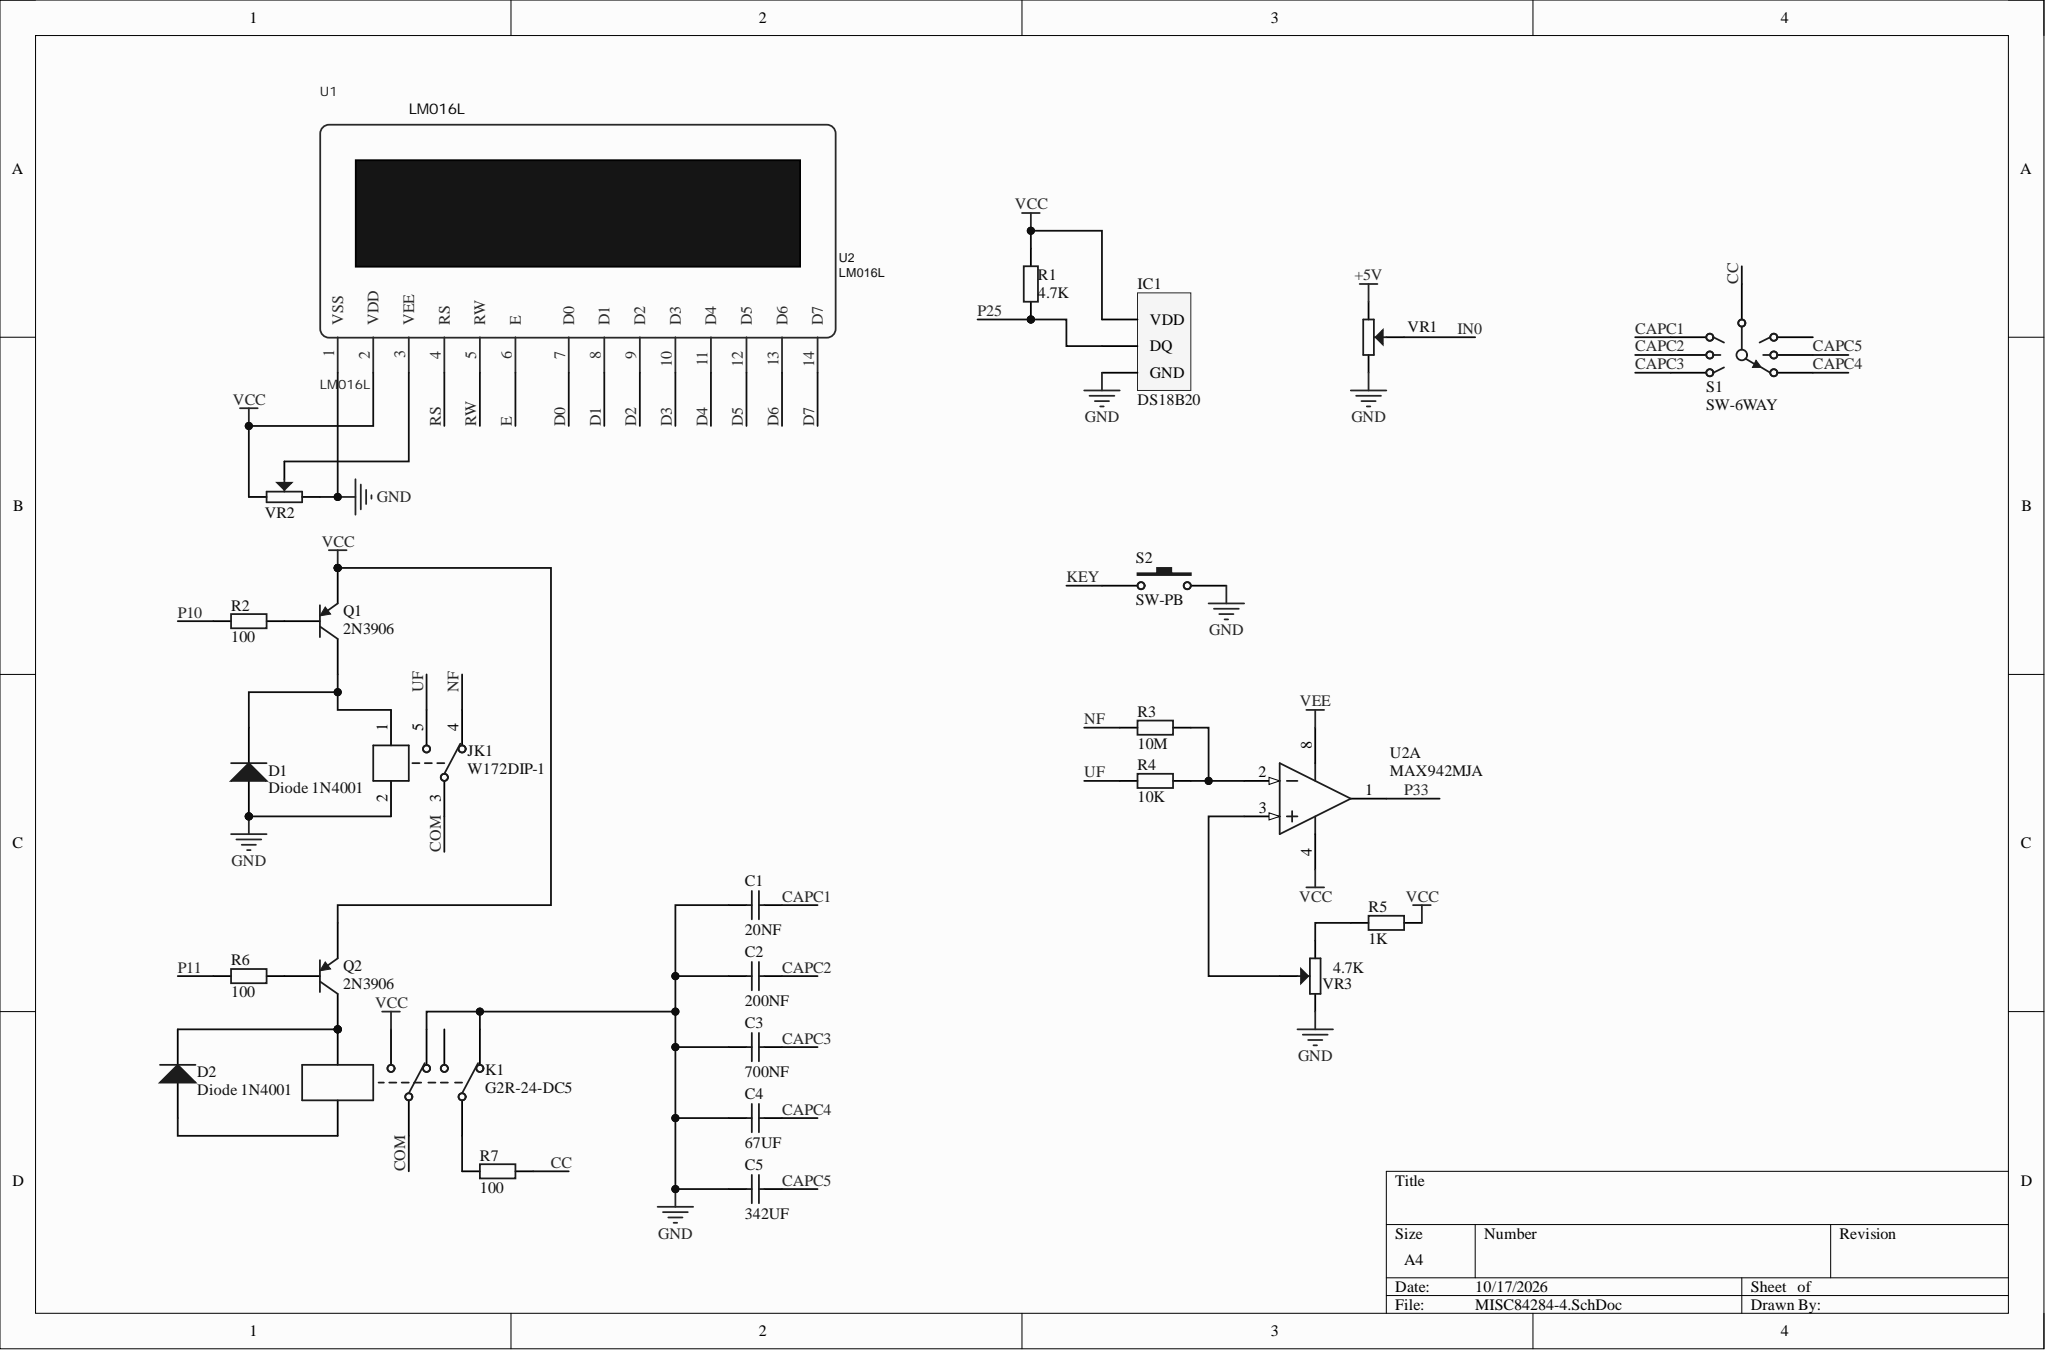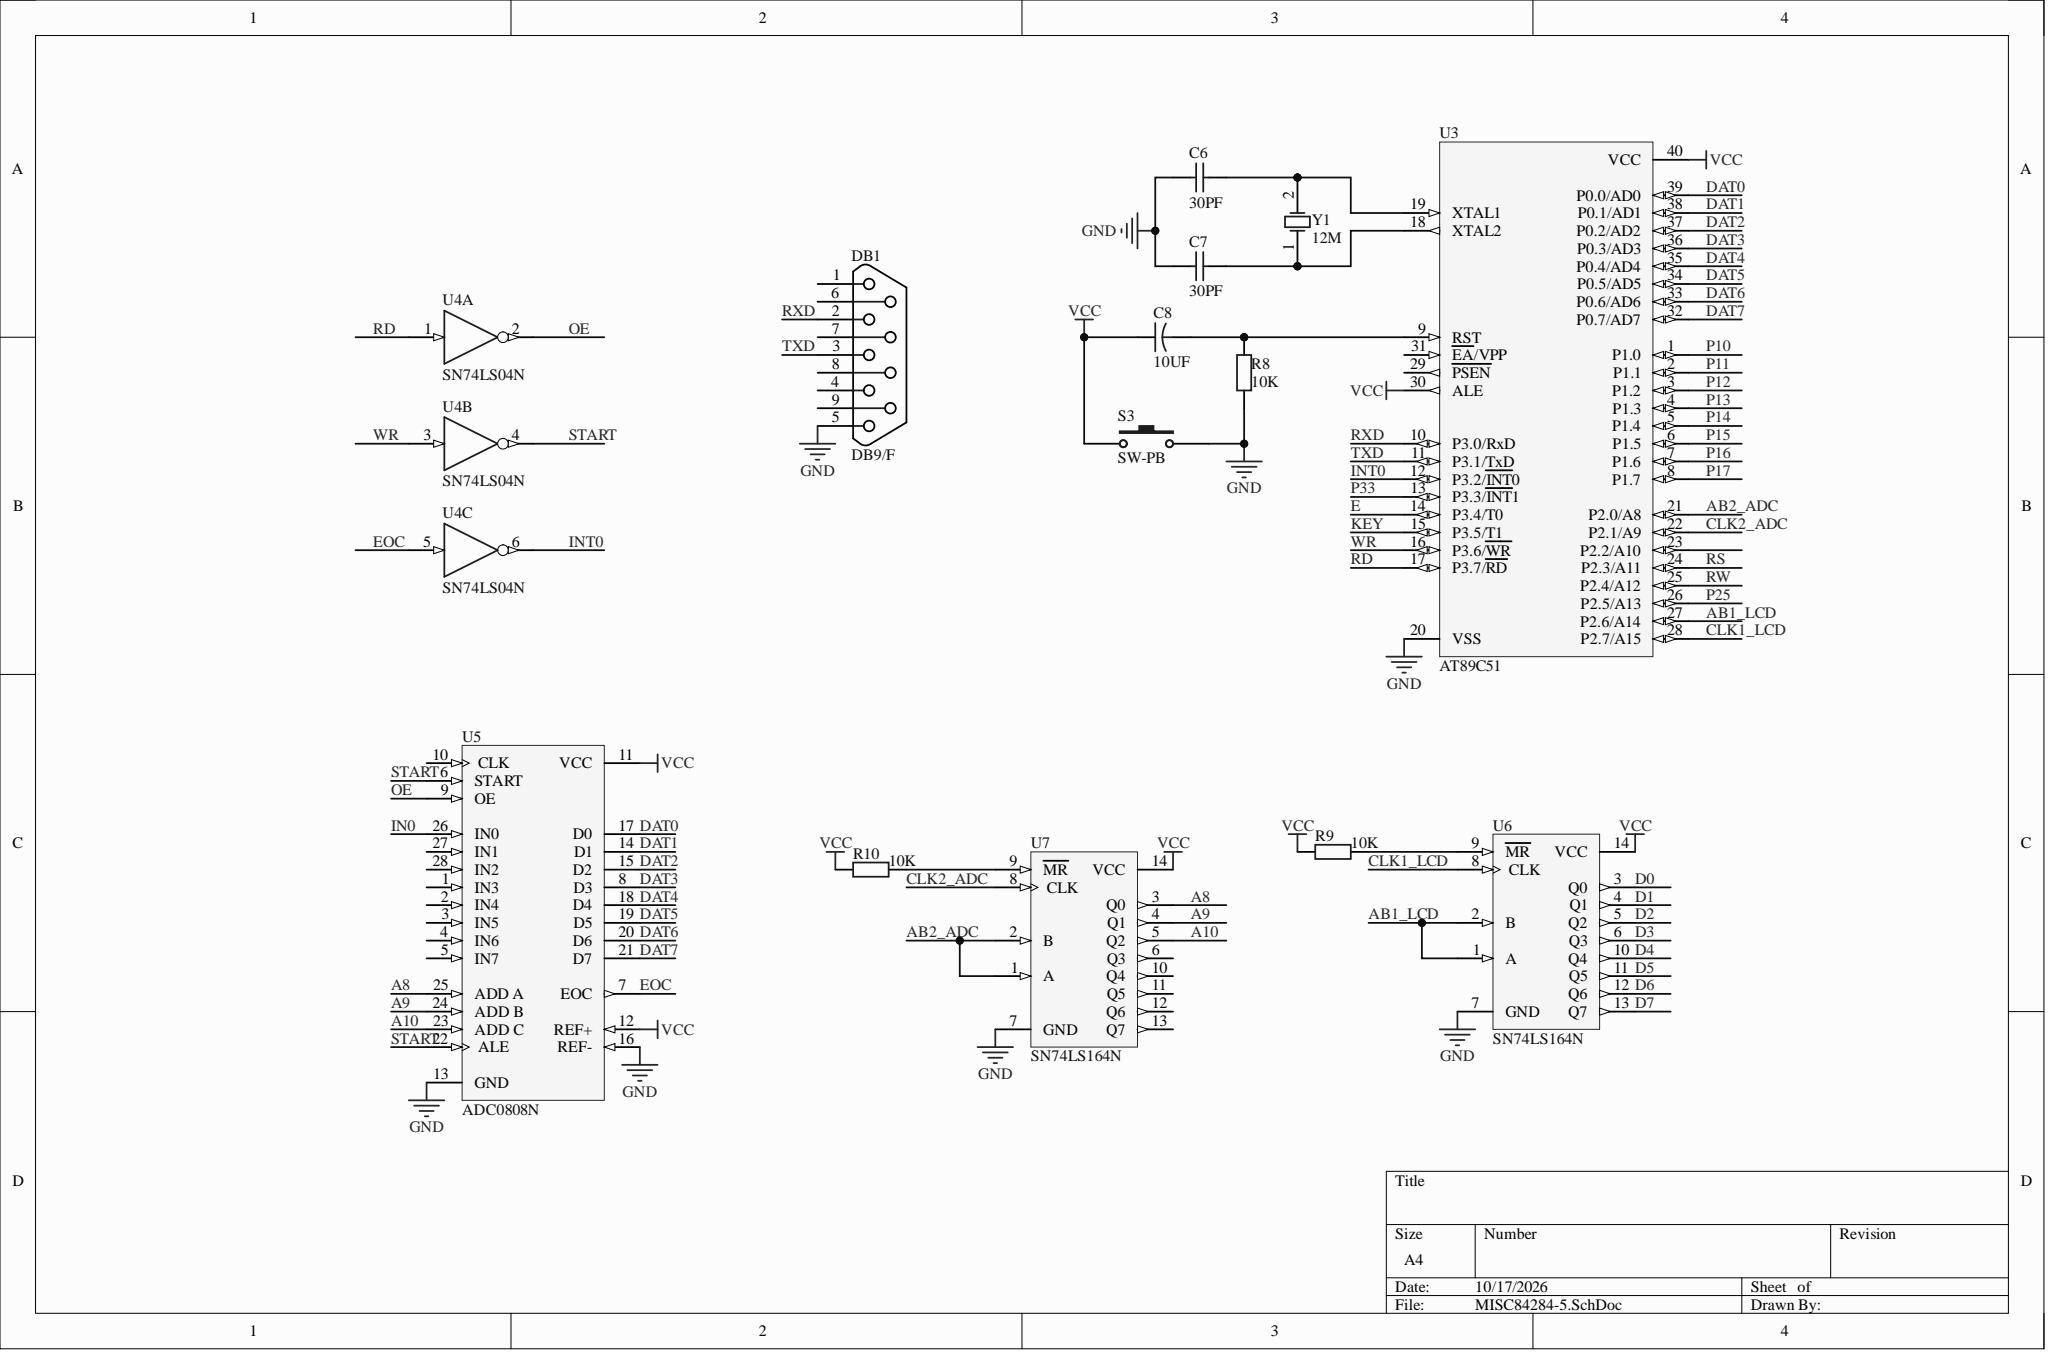Circuit board | Altium Designer | 40 parts | 66 nets
Bill of materials:
Comment,Description,Designator,Footprint,LibRef,Quantity
"20NF","Capacitor","C1","RAD-0.2","Cap","1"
"200NF","Capacitor","C2","RAD-0.2","Cap","1"
"700NF","Capacitor","C3","RAD-0.2","Cap","1"
"67UF","Capacitor","C4","RAD-0.2","Cap","1"
"342UF","Capacitor","C5","RAD-0.2","Cap","1"
"30PF","Capacitor","C6, C7","RAD-0.2","Cap","2"
"10UF","Capacitor","C8","CAPR5-4X5","Cap2","1"
"Diode 1N4001","1 Amp General Purpose Rectifier","D1, D2","DO-41","Diode 1N4001","2"
"DB9/F","","DB1","DB9/F/180","DB9/F","1"
"DS18B20","Digital thermometer","IC1","HDR1X3","DS18B20","1"
"W172DIP-1","","JK1","SRD-C_BK","SRD-S-105D","1"
"G2R-24-DC5","Dual-Pole Dual-Throw Relay","K1","DIP-P8","Relay-DPDT","1"
"2N3906","PNP General Purpose Amplifier","Q1, Q2","TO-92A","2N3906","2"
"4.7K","Resistor","R1","AXIAL-0.4","Res2","1"
"100","Resistor","R2, R6, R7","AXIAL-0.4","Res2","3"
"10M","Resistor","R3","AXIAL-0.4","Res2","1"
"10K","Resistor","R4, R8, R9, R10","AXIAL-0.4","Res2","4"
"1K","Resistor","R5","AXIAL-0.4","Res2","1"
"SW-6WAY","6 Way Switch","S1","SW-7","SW-6WAY","1"
"SW-PB","Switch","S2, S3","SPST-2","SW-PB","2"
"LM016L","","U1","LM016L","LM016L","1"
"MAX942MJA","High-speed, Low-power, 3V/5V, Rail-to-Rail Dual-Supply Comparator","U2","JA8","MAX942MJA","1"
"AT89C51","51 series MCU","U3","DIP40","AT89C51","1"
"SN74LS04N","Hex Inverter","U4","646-06","SN74LS04N","1"
"ADC0808N","CMOS Analog-to-Digital Converter with 8-Channel Multiplexer","U5","N028","ADC0808N","1"
"SN74LS164N","Serial-In Parallel-Out Shift Register","U6, U7","646-06","SN74LS164N","2"
"RESVR","","VR1, VR2","3296W","RESVR","2"
"4.7K","","VR3","3296W","RESVR","1"
"12M","Crystal Oscillator","Y1","XTAL_US","XTAL","1"
Netlist (Protel format):
[
C1
RAD-0.2
20NF



]
[
C2
RAD-0.2
200NF



]
[
C3
RAD-0.2
700NF



]
[
C4
RAD-0.2
67UF



]
[
C5
RAD-0.2
342UF



]
[
C6
RAD-0.2
30PF



]
[
C7
RAD-0.2
30PF



]
[
C8
CAPR5-4X5
10UF



]
[
D1
DO-41
Diode 1N4001



]
[
D2
DO-41
Diode 1N4001



]
[
DB1
DB9/F/180
DB9/F



]
[
IC1
HDR1X3
DS18B20



]
[
JK1
SRD-C_BK
W172DIP-1



]
[
K1
DIP-P8
G2R-24-DC5



]
[
Q1
TO-92A
2N3906



]
[
Q2
TO-92A
2N3906



]
[
R1
AXIAL-0.4
4.7K



]
[
R2
AXIAL-0.4
100



]
[
R3
AXIAL-0.4
10M



]
[
R4
AXIAL-0.4
10K



]
[
R5
AXIAL-0.4
1K



]
[
R6
AXIAL-0.4
100



]
[
R7
AXIAL-0.4
100



]
[
R8
AXIAL-0.4
10K



]
[
R9
AXIAL-0.4
10K



]
[
R10
AXIAL-0.4
10K



]
[
S1
SW-7
SW-6WAY



]
[
S2
SPST-2
SW-PB



]
[
S3
SPST-2
SW-PB



]
[
U1
LM016L
LM016L



]
[
U2
JA8
MAX942MJA



]
[
U3
DIP40
AT89C51



]
[
U4
646-06
SN74LS04N



]
[
U5
N028
ADC0808N



]
[
U6
646-06
SN74LS164N



]
[
U7
646-06
SN74LS164N



]
[
VR1
3296W
RESVR



]
[
VR2
3296W
RESVR



]
[
VR3
3296W
4.7K



]
[
Y1
XTAL_US
12M



]
(
WR
U3-16
U4-3
)
(
VCC
C8-1
IC1-3
K1-6
Q1-1
Q2-1
R1-2
R5-1
R9-2
R10-2
S3-1
U1-2
U2-4
U3-30
U3-40
U5-11
U5-12
U6-14
U7-14
VR2-1
)
(
UF
JK1-5
R4-2
)
(
TXD
DB1-3
U3-11
)
(
START
U4-4
U5-6
U5-22
)
(
RXD
DB1-2
U3-10
)
(
RW
U1-5
U3-25
)
(
RS
U1-4
U3-24
)
(
RD
U3-17
U4-1
)
(
P33
U2-1
U3-13
)
(
P25
IC1-2
R1-1
U3-26
)
(
P11
R6-2
U3-2
)
(
P10
R2-2
U3-1
)
(
OE
U4-2
U5-9
)
(
NF
JK1-4
R3-2
)
(
NetU2_3
U2-3
VR3-2
)
(
NetU1_3
U1-3
VR2-2
)
(
NetR10_1
R10-1
U7-9
)
(
NetR9_1
R9-1
U6-9
)
(
NetR5_2
R5-2
VR3-2
)
(
NetR3_1
R3-1
R4-1
U2-2
)
(
NetQ2_2
Q2-2
R6-1
)
(
NetQ1_2
Q1-2
R2-1
)
(
NetK1_1
K1-1
R7-2
)
(
NetD2_2
D2-2
K1-8
Q2-3
)
(
NetD2_1
D2-1
K1-7
)
(
NetD1_2
D1-2
JK1-1
Q1-3
)
(
NetC8_2
C8-2
R8-2
U3-9
)
(
NetC7_2
C7-2
U3-18
Y1-1
)
(
NetC6_2
C6-2
U3-19
Y1-2
)
(
KEY
S2-1
U3-15
)
(
INT0
U3-12
U4-6
)
(
IN0
U5-26
VR1-2
)
(
GND
C1-1
C2-1
C3-1
C4-1
C5-1
C6-1
C7-1
D1-1
DB1-5
IC1-1
JK1-2
K1-2
K1-5
R8-1
S2-2
S3-2
U1-1
U3-20
U4-7
U5-13
U5-16
U6-7
U7-7
VR1-2
VR2-2
VR3-1
)
(
EOC
U4-5
U5-7
)
(
E
U1-6
U3-14
)
(
DAT7
U3-32
U5-21
)
(
DAT6
U3-33
U5-20
)
(
DAT5
U3-34
U5-19
)
(
DAT4
U3-35
U5-18
)
(
DAT3
U3-36
U5-8
)
(
DAT2
U3-37
U5-15
)
(
DAT1
U3-38
U5-14
)
(
DAT0
U3-39
U5-17
)
(
D7
U1-14
U6-13
)
(
D6
U1-13
U6-12
)
(
D5
U1-12
U6-11
)
(
D4
U1-11
U6-10
)
(
D3
U1-10
U6-6
)
(
D2
U1-9
U6-5
)
(
D1
U1-8
U6-4
)
(
D0
U1-7
U6-3
)
(
COM
JK1-3
K1-4
)
(
CLK2_ADC
U3-22
U7-8
)
(
CLK1_LCD
U3-28
U6-8
)
(
CC
R7-1
S1-7
)
(
CAPC5
C5-2
S1-5
)
(
CAPC4
C4-2
S1-6
)
(
CAPC3
C3-2
S1-3
)
(
CAPC2
C2-2
S1-2
)
(
CAPC1
C1-2
S1-1
)
(
AB2_ADC
U3-21
U7-1
U7-2
)
(
AB1_LCD
U3-27
U6-1
U6-2
)
(
A10
U5-23
U7-5
)
(
A9
U5-24
U7-4
)
(
A8
U5-25
U7-3
)